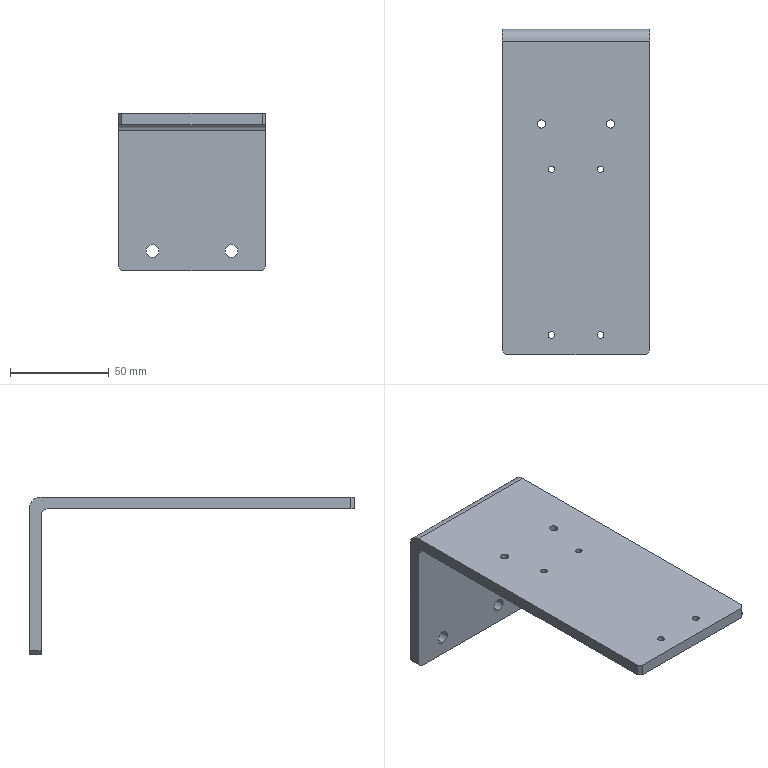Part | SolidWorks | features HoleWzd 3, Fillet 2, Chamfer 1, Extrusion 1, Shell 1 | 1 solid | 30 faces | box 75 x 165 x 80 mm | volume 106298 mm3 | cylinder 18 | plane 12 | commonest cylinder face diameters 3.3 x8 4.2 x4 6.5 x4 6 x1 12 x1
STEP:
#1=CARTESIAN_POINT('',(19.6,34.5,80.));
#2=VERTEX_POINT('',#1);
#3=CARTESIAN_POINT('',(15.4,34.5,80.));
#4=VERTEX_POINT('',#3);
#5=CARTESIAN_POINT('',(17.5,34.5,80.));
#6=DIRECTION('',(0.,0.,-1.));
#7=DIRECTION('',(-1.,0.,0.));
#8=AXIS2_PLACEMENT_3D('',#5,#6,#7);
#9=CIRCLE('',#8,2.1);
#10=EDGE_CURVE('',#2,#4,#9,.T.);
#11=ORIENTED_EDGE('',*,*,#10,.F.);
#12=CARTESIAN_POINT('',(19.6,34.5,74.));
#13=VERTEX_POINT('',#12);
#14=CARTESIAN_POINT('',(19.6,34.5,74.));
#15=DIRECTION('',(0.,0.,-1.));
#16=VECTOR('',#15,1000.);
#17=LINE('',#14,#16);
#18=EDGE_CURVE('',#2,#13,#17,.T.);
#19=ORIENTED_EDGE('',*,*,#18,.T.);
#20=CARTESIAN_POINT('',(15.4,34.5,74.));
#21=VERTEX_POINT('',#20);
#22=CARTESIAN_POINT('',(17.5,34.5,74.));
#23=DIRECTION('',(0.,0.,-1.));
#24=DIRECTION('',(-1.,0.,0.));
#25=AXIS2_PLACEMENT_3D('',#22,#23,#24);
#26=CIRCLE('',#25,2.1);
#27=EDGE_CURVE('',#13,#21,#26,.T.);
#28=ORIENTED_EDGE('',*,*,#27,.T.);
#29=CARTESIAN_POINT('',(15.4,34.5,74.));
#30=DIRECTION('',(0.,0.,-1.));
#31=VECTOR('',#30,1000.);
#32=LINE('',#29,#31);
#33=EDGE_CURVE('',#4,#21,#32,.T.);
#34=ORIENTED_EDGE('',*,*,#33,.F.);
#35=EDGE_LOOP('',(#11,#19,#28,#34));
#36=FACE_OUTER_BOUND('',#35,.T.);
#37=CARTESIAN_POINT('',(17.5,34.5,74.));
#38=DIRECTION('',(0.,0.,-1.));
#39=DIRECTION('',(-1.,0.,0.));
#40=AXIS2_PLACEMENT_3D('',#37,#38,#39);
#41=CYLINDRICAL_SURFACE('',#40,2.1);
#42=ADVANCED_FACE('',(#36),#41,.F.);
#43=CARTESIAN_POINT('',(-15.4,34.5,80.));
#44=VERTEX_POINT('',#43);
#45=CARTESIAN_POINT('',(-19.6,34.5,80.));
#46=VERTEX_POINT('',#45);
#47=CARTESIAN_POINT('',(-17.5,34.5,80.));
#48=DIRECTION('',(0.,0.,-1.));
#49=DIRECTION('',(-1.,0.,0.));
#50=AXIS2_PLACEMENT_3D('',#47,#48,#49);
#51=CIRCLE('',#50,2.1);
#52=EDGE_CURVE('',#44,#46,#51,.T.);
#53=ORIENTED_EDGE('',*,*,#52,.F.);
#54=CARTESIAN_POINT('',(-15.4,34.5,74.));
#55=VERTEX_POINT('',#54);
#56=CARTESIAN_POINT('',(-15.4,34.5,74.));
#57=DIRECTION('',(0.,0.,-1.));
#58=VECTOR('',#57,1000.);
#59=LINE('',#56,#58);
#60=EDGE_CURVE('',#44,#55,#59,.T.);
#61=ORIENTED_EDGE('',*,*,#60,.T.);
#62=CARTESIAN_POINT('',(-19.6,34.5,74.));
#63=VERTEX_POINT('',#62);
#64=CARTESIAN_POINT('',(-17.5,34.5,74.));
#65=DIRECTION('',(0.,0.,-1.));
#66=DIRECTION('',(-1.,0.,0.));
#67=AXIS2_PLACEMENT_3D('',#64,#65,#66);
#68=CIRCLE('',#67,2.1);
#69=EDGE_CURVE('',#55,#63,#68,.T.);
#70=ORIENTED_EDGE('',*,*,#69,.T.);
#71=CARTESIAN_POINT('',(-19.6,34.5,74.));
#72=DIRECTION('',(0.,0.,-1.));
#73=VECTOR('',#72,1000.);
#74=LINE('',#71,#73);
#75=EDGE_CURVE('',#46,#63,#74,.T.);
#76=ORIENTED_EDGE('',*,*,#75,.F.);
#77=EDGE_LOOP('',(#53,#61,#70,#76));
#78=FACE_OUTER_BOUND('',#77,.T.);
#79=CARTESIAN_POINT('',(-17.5,34.5,74.));
#80=DIRECTION('',(0.,0.,-1.));
#81=DIRECTION('',(-1.,0.,0.));
#82=AXIS2_PLACEMENT_3D('',#79,#80,#81);
#83=CYLINDRICAL_SURFACE('',#82,2.1);
#84=ADVANCED_FACE('',(#78),#83,.F.);
#85=CARTESIAN_POINT('',(-20.,82.5,13.25));
#86=VERTEX_POINT('',#85);
#87=CARTESIAN_POINT('',(-20.,82.5,6.75));
#88=VERTEX_POINT('',#87);
#89=CARTESIAN_POINT('',(-20.,82.5,10.));
#90=DIRECTION('',(0.,-1.,0.));
#91=DIRECTION('',(0.,0.,-1.));
#92=AXIS2_PLACEMENT_3D('',#89,#90,#91);
#93=CIRCLE('',#92,3.25);
#94=EDGE_CURVE('',#86,#88,#93,.T.);
#95=ORIENTED_EDGE('',*,*,#94,.F.);
#96=CARTESIAN_POINT('',(-20.,76.5,13.25));
#97=VERTEX_POINT('',#96);
#98=CARTESIAN_POINT('',(-20.,76.5,13.25));
#99=DIRECTION('',(0.,-1.,0.));
#100=VECTOR('',#99,1000.);
#101=LINE('',#98,#100);
#102=EDGE_CURVE('',#86,#97,#101,.T.);
#103=ORIENTED_EDGE('',*,*,#102,.T.);
#104=CARTESIAN_POINT('',(-20.,76.5,6.75));
#105=VERTEX_POINT('',#104);
#106=CARTESIAN_POINT('',(-20.,76.5,10.));
#107=DIRECTION('',(0.,-1.,0.));
#108=DIRECTION('',(0.,0.,-1.));
#109=AXIS2_PLACEMENT_3D('',#106,#107,#108);
#110=CIRCLE('',#109,3.25);
#111=EDGE_CURVE('',#97,#105,#110,.T.);
#112=ORIENTED_EDGE('',*,*,#111,.T.);
#113=CARTESIAN_POINT('',(-20.,76.5,6.75));
#114=DIRECTION('',(0.,-1.,0.));
#115=VECTOR('',#114,1000.);
#116=LINE('',#113,#115);
#117=EDGE_CURVE('',#88,#105,#116,.T.);
#118=ORIENTED_EDGE('',*,*,#117,.F.);
#119=EDGE_LOOP('',(#95,#103,#112,#118));
#120=FACE_OUTER_BOUND('',#119,.T.);
#121=CARTESIAN_POINT('',(-20.,76.5,10.));
#122=DIRECTION('',(0.,-1.,0.));
#123=DIRECTION('',(0.,0.,-1.));
#124=AXIS2_PLACEMENT_3D('',#121,#122,#123);
#125=CYLINDRICAL_SURFACE('',#124,3.25);
#126=ADVANCED_FACE('',(#120),#125,.F.);
#127=CARTESIAN_POINT('',(20.,82.5,13.25));
#128=VERTEX_POINT('',#127);
#129=CARTESIAN_POINT('',(20.,82.5,6.75));
#130=VERTEX_POINT('',#129);
#131=CARTESIAN_POINT('',(20.,82.5,10.));
#132=DIRECTION('',(0.,-1.,0.));
#133=DIRECTION('',(0.,0.,-1.));
#134=AXIS2_PLACEMENT_3D('',#131,#132,#133);
#135=CIRCLE('',#134,3.25);
#136=EDGE_CURVE('',#128,#130,#135,.T.);
#137=ORIENTED_EDGE('',*,*,#136,.F.);
#138=CARTESIAN_POINT('',(20.,76.5,13.25));
#139=VERTEX_POINT('',#138);
#140=CARTESIAN_POINT('',(20.,76.5,13.25));
#141=DIRECTION('',(0.,-1.,0.));
#142=VECTOR('',#141,1000.);
#143=LINE('',#140,#142);
#144=EDGE_CURVE('',#128,#139,#143,.T.);
#145=ORIENTED_EDGE('',*,*,#144,.T.);
#146=CARTESIAN_POINT('',(20.,76.5,6.75));
#147=VERTEX_POINT('',#146);
#148=CARTESIAN_POINT('',(20.,76.5,10.));
#149=DIRECTION('',(0.,-1.,0.));
#150=DIRECTION('',(0.,0.,-1.));
#151=AXIS2_PLACEMENT_3D('',#148,#149,#150);
#152=CIRCLE('',#151,3.25);
#153=EDGE_CURVE('',#139,#147,#152,.T.);
#154=ORIENTED_EDGE('',*,*,#153,.T.);
#155=CARTESIAN_POINT('',(20.,76.5,6.75));
#156=DIRECTION('',(0.,-1.,0.));
#157=VECTOR('',#156,1000.);
#158=LINE('',#155,#157);
#159=EDGE_CURVE('',#130,#147,#158,.T.);
#160=ORIENTED_EDGE('',*,*,#159,.F.);
#161=EDGE_LOOP('',(#137,#145,#154,#160));
#162=FACE_OUTER_BOUND('',#161,.T.);
#163=CARTESIAN_POINT('',(20.,76.5,10.));
#164=DIRECTION('',(0.,-1.,0.));
#165=DIRECTION('',(0.,0.,-1.));
#166=AXIS2_PLACEMENT_3D('',#163,#164,#165);
#167=CYLINDRICAL_SURFACE('',#166,3.25);
#168=ADVANCED_FACE('',(#162),#167,.F.);
#169=CARTESIAN_POINT('',(14.15,-72.5,80.));
#170=VERTEX_POINT('',#169);
#171=CARTESIAN_POINT('',(10.85,-72.5,80.));
#172=VERTEX_POINT('',#171);
#173=CARTESIAN_POINT('',(12.5,-72.5,80.));
#174=DIRECTION('',(0.,0.,-1.));
#175=DIRECTION('',(-1.,0.,0.));
#176=AXIS2_PLACEMENT_3D('',#173,#174,#175);
#177=CIRCLE('',#176,1.65);
#178=EDGE_CURVE('',#170,#172,#177,.T.);
#179=ORIENTED_EDGE('',*,*,#178,.F.);
#180=CARTESIAN_POINT('',(14.15,-72.5,74.));
#181=VERTEX_POINT('',#180);
#182=CARTESIAN_POINT('',(14.15,-72.5,74.));
#183=DIRECTION('',(0.,0.,-1.));
#184=VECTOR('',#183,1000.);
#185=LINE('',#182,#184);
#186=EDGE_CURVE('',#170,#181,#185,.T.);
#187=ORIENTED_EDGE('',*,*,#186,.T.);
#188=CARTESIAN_POINT('',(10.85,-72.5,74.));
#189=VERTEX_POINT('',#188);
#190=CARTESIAN_POINT('',(12.5,-72.5,74.));
#191=DIRECTION('',(0.,0.,-1.));
#192=DIRECTION('',(-1.,0.,0.));
#193=AXIS2_PLACEMENT_3D('',#190,#191,#192);
#194=CIRCLE('',#193,1.65);
#195=EDGE_CURVE('',#181,#189,#194,.T.);
#196=ORIENTED_EDGE('',*,*,#195,.T.);
#197=CARTESIAN_POINT('',(10.85,-72.5,74.));
#198=DIRECTION('',(0.,0.,-1.));
#199=VECTOR('',#198,1000.);
#200=LINE('',#197,#199);
#201=EDGE_CURVE('',#172,#189,#200,.T.);
#202=ORIENTED_EDGE('',*,*,#201,.F.);
#203=EDGE_LOOP('',(#179,#187,#196,#202));
#204=FACE_OUTER_BOUND('',#203,.T.);
#205=CARTESIAN_POINT('',(12.5,-72.5,74.));
#206=DIRECTION('',(0.,0.,-1.));
#207=DIRECTION('',(-1.,0.,0.));
#208=AXIS2_PLACEMENT_3D('',#205,#206,#207);
#209=CYLINDRICAL_SURFACE('',#208,1.65);
#210=ADVANCED_FACE('',(#204),#209,.F.);
#211=CARTESIAN_POINT('',(14.15,11.5,80.));
#212=VERTEX_POINT('',#211);
#213=CARTESIAN_POINT('',(10.85,11.5,80.));
#214=VERTEX_POINT('',#213);
#215=CARTESIAN_POINT('',(12.5,11.5,80.));
#216=DIRECTION('',(0.,0.,-1.));
#217=DIRECTION('',(-1.,0.,0.));
#218=AXIS2_PLACEMENT_3D('',#215,#216,#217);
#219=CIRCLE('',#218,1.65);
#220=EDGE_CURVE('',#212,#214,#219,.T.);
#221=ORIENTED_EDGE('',*,*,#220,.F.);
#222=CARTESIAN_POINT('',(14.15,11.5,74.));
#223=VERTEX_POINT('',#222);
#224=CARTESIAN_POINT('',(14.15,11.5,74.));
#225=DIRECTION('',(0.,0.,-1.));
#226=VECTOR('',#225,1000.);
#227=LINE('',#224,#226);
#228=EDGE_CURVE('',#212,#223,#227,.T.);
#229=ORIENTED_EDGE('',*,*,#228,.T.);
#230=CARTESIAN_POINT('',(10.85,11.5,74.));
#231=VERTEX_POINT('',#230);
#232=CARTESIAN_POINT('',(12.5,11.5,74.));
#233=DIRECTION('',(0.,0.,-1.));
#234=DIRECTION('',(-1.,0.,0.));
#235=AXIS2_PLACEMENT_3D('',#232,#233,#234);
#236=CIRCLE('',#235,1.65);
#237=EDGE_CURVE('',#223,#231,#236,.T.);
#238=ORIENTED_EDGE('',*,*,#237,.T.);
#239=CARTESIAN_POINT('',(10.85,11.5,74.));
#240=DIRECTION('',(0.,0.,-1.));
#241=VECTOR('',#240,1000.);
#242=LINE('',#239,#241);
#243=EDGE_CURVE('',#214,#231,#242,.T.);
#244=ORIENTED_EDGE('',*,*,#243,.F.);
#245=EDGE_LOOP('',(#221,#229,#238,#244));
#246=FACE_OUTER_BOUND('',#245,.T.);
#247=CARTESIAN_POINT('',(12.5,11.5,74.));
#248=DIRECTION('',(0.,0.,-1.));
#249=DIRECTION('',(-1.,0.,0.));
#250=AXIS2_PLACEMENT_3D('',#247,#248,#249);
#251=CYLINDRICAL_SURFACE('',#250,1.65);
#252=ADVANCED_FACE('',(#246),#251,.F.);
#253=CARTESIAN_POINT('',(-10.85,11.5,80.));
#254=VERTEX_POINT('',#253);
#255=CARTESIAN_POINT('',(-14.15,11.5,80.));
#256=VERTEX_POINT('',#255);
#257=CARTESIAN_POINT('',(-12.5,11.5,80.));
#258=DIRECTION('',(0.,0.,-1.));
#259=DIRECTION('',(-1.,0.,0.));
#260=AXIS2_PLACEMENT_3D('',#257,#258,#259);
#261=CIRCLE('',#260,1.65);
#262=EDGE_CURVE('',#254,#256,#261,.T.);
#263=ORIENTED_EDGE('',*,*,#262,.F.);
#264=CARTESIAN_POINT('',(-10.85,11.5,74.));
#265=VERTEX_POINT('',#264);
#266=CARTESIAN_POINT('',(-10.85,11.5,74.));
#267=DIRECTION('',(0.,0.,-1.));
#268=VECTOR('',#267,1000.);
#269=LINE('',#266,#268);
#270=EDGE_CURVE('',#254,#265,#269,.T.);
#271=ORIENTED_EDGE('',*,*,#270,.T.);
#272=CARTESIAN_POINT('',(-14.15,11.5,74.));
#273=VERTEX_POINT('',#272);
#274=CARTESIAN_POINT('',(-12.5,11.5,74.));
#275=DIRECTION('',(0.,0.,-1.));
#276=DIRECTION('',(-1.,0.,0.));
#277=AXIS2_PLACEMENT_3D('',#274,#275,#276);
#278=CIRCLE('',#277,1.65);
#279=EDGE_CURVE('',#265,#273,#278,.T.);
#280=ORIENTED_EDGE('',*,*,#279,.T.);
#281=CARTESIAN_POINT('',(-14.15,11.5,74.));
#282=DIRECTION('',(0.,0.,-1.));
#283=VECTOR('',#282,1000.);
#284=LINE('',#281,#283);
#285=EDGE_CURVE('',#256,#273,#284,.T.);
#286=ORIENTED_EDGE('',*,*,#285,.F.);
#287=EDGE_LOOP('',(#263,#271,#280,#286));
#288=FACE_OUTER_BOUND('',#287,.T.);
#289=CARTESIAN_POINT('',(-12.5,11.5,74.));
#290=DIRECTION('',(0.,0.,-1.));
#291=DIRECTION('',(-1.,0.,0.));
#292=AXIS2_PLACEMENT_3D('',#289,#290,#291);
#293=CYLINDRICAL_SURFACE('',#292,1.65);
#294=ADVANCED_FACE('',(#288),#293,.F.);
#295=CARTESIAN_POINT('',(-10.85,-72.5,80.));
#296=VERTEX_POINT('',#295);
#297=CARTESIAN_POINT('',(-14.15,-72.5,80.));
#298=VERTEX_POINT('',#297);
#299=CARTESIAN_POINT('',(-12.5,-72.5,80.));
#300=DIRECTION('',(0.,0.,-1.));
#301=DIRECTION('',(-1.,0.,0.));
#302=AXIS2_PLACEMENT_3D('',#299,#300,#301);
#303=CIRCLE('',#302,1.65);
#304=EDGE_CURVE('',#296,#298,#303,.T.);
#305=ORIENTED_EDGE('',*,*,#304,.F.);
#306=CARTESIAN_POINT('',(-10.85,-72.5,74.));
#307=VERTEX_POINT('',#306);
#308=CARTESIAN_POINT('',(-10.85,-72.5,74.));
#309=DIRECTION('',(0.,0.,-1.));
#310=VECTOR('',#309,1000.);
#311=LINE('',#308,#310);
#312=EDGE_CURVE('',#296,#307,#311,.T.);
#313=ORIENTED_EDGE('',*,*,#312,.T.);
#314=CARTESIAN_POINT('',(-14.15,-72.5,74.));
#315=VERTEX_POINT('',#314);
#316=CARTESIAN_POINT('',(-12.5,-72.5,74.));
#317=DIRECTION('',(0.,0.,-1.));
#318=DIRECTION('',(-1.,0.,0.));
#319=AXIS2_PLACEMENT_3D('',#316,#317,#318);
#320=CIRCLE('',#319,1.65);
#321=EDGE_CURVE('',#307,#315,#320,.T.);
#322=ORIENTED_EDGE('',*,*,#321,.T.);
#323=CARTESIAN_POINT('',(-14.15,-72.5,74.));
#324=DIRECTION('',(0.,0.,-1.));
#325=VECTOR('',#324,1000.);
#326=LINE('',#323,#325);
#327=EDGE_CURVE('',#298,#315,#326,.T.);
#328=ORIENTED_EDGE('',*,*,#327,.F.);
#329=EDGE_LOOP('',(#305,#313,#322,#328));
#330=FACE_OUTER_BOUND('',#329,.T.);
#331=CARTESIAN_POINT('',(-12.5,-72.5,74.));
#332=DIRECTION('',(0.,0.,-1.));
#333=DIRECTION('',(-1.,0.,0.));
#334=AXIS2_PLACEMENT_3D('',#331,#332,#333);
#335=CYLINDRICAL_SURFACE('',#334,1.65);
#336=ADVANCED_FACE('',(#330),#335,.F.);
#337=CARTESIAN_POINT('',(37.5,-80.5,80.));
#338=VERTEX_POINT('',#337);
#339=CARTESIAN_POINT('',(37.5,76.5,80.));
#340=VERTEX_POINT('',#339);
#341=CARTESIAN_POINT('',(37.5,82.5,80.));
#342=DIRECTION('',(0.,1.,0.));
#343=VECTOR('',#342,1000.);
#344=LINE('',#341,#343);
#345=EDGE_CURVE('',#338,#340,#344,.T.);
#346=ORIENTED_EDGE('',*,*,#345,.F.);
#347=CARTESIAN_POINT('',(37.5,-80.5,74.));
#348=VERTEX_POINT('',#347);
#349=CARTESIAN_POINT('',(37.5,-80.5,80.));
#350=DIRECTION('',(0.,0.,-1.));
#351=VECTOR('',#350,1000.);
#352=LINE('',#349,#351);
#353=EDGE_CURVE('',#338,#348,#352,.T.);
#354=ORIENTED_EDGE('',*,*,#353,.T.);
#355=CARTESIAN_POINT('',(37.5,73.5,74.));
#356=VERTEX_POINT('',#355);
#357=CARTESIAN_POINT('',(37.5,82.5,74.));
#358=DIRECTION('',(0.,1.,0.));
#359=VECTOR('',#358,1000.);
#360=LINE('',#357,#359);
#361=EDGE_CURVE('',#348,#356,#360,.T.);
#362=ORIENTED_EDGE('',*,*,#361,.T.);
#363=CARTESIAN_POINT('',(37.5,76.5,71.));
#364=VERTEX_POINT('',#363);
#365=CARTESIAN_POINT('',(37.5,73.5,71.));
#366=DIRECTION('',(-1.,0.,0.));
#367=DIRECTION('',(0.,-1.,0.));
#368=AXIS2_PLACEMENT_3D('',#365,#366,#367);
#369=CIRCLE('',#368,3.);
#370=EDGE_CURVE('',#356,#364,#369,.T.);
#371=ORIENTED_EDGE('',*,*,#370,.T.);
#372=CARTESIAN_POINT('',(37.5,76.5,2.));
#373=VERTEX_POINT('',#372);
#374=CARTESIAN_POINT('',(37.5,76.5,80.));
#375=DIRECTION('',(0.,0.,-1.));
#376=VECTOR('',#375,1000.);
#377=LINE('',#374,#376);
#378=EDGE_CURVE('',#364,#373,#377,.T.);
#379=ORIENTED_EDGE('',*,*,#378,.T.);
#380=CARTESIAN_POINT('',(37.5,82.5,2.));
#381=VERTEX_POINT('',#380);
#382=CARTESIAN_POINT('',(37.5,82.5,2.));
#383=DIRECTION('',(0.,1.,0.));
#384=VECTOR('',#383,1000.);
#385=LINE('',#382,#384);
#386=EDGE_CURVE('',#373,#381,#385,.T.);
#387=ORIENTED_EDGE('',*,*,#386,.T.);
#388=CARTESIAN_POINT('',(37.5,82.5,74.));
#389=VERTEX_POINT('',#388);
#390=CARTESIAN_POINT('',(37.5,82.5,80.));
#391=DIRECTION('',(0.,0.,-1.));
#392=VECTOR('',#391,1000.);
#393=LINE('',#390,#392);
#394=EDGE_CURVE('',#389,#381,#393,.T.);
#395=ORIENTED_EDGE('',*,*,#394,.F.);
#396=CARTESIAN_POINT('',(37.5,76.5,74.));
#397=DIRECTION('',(1.,0.,0.));
#398=DIRECTION('',(0.,-1.,0.));
#399=AXIS2_PLACEMENT_3D('',#396,#397,#398);
#400=CIRCLE('',#399,6.);
#401=EDGE_CURVE('',#389,#340,#400,.T.);
#402=ORIENTED_EDGE('',*,*,#401,.T.);
#403=EDGE_LOOP('',(#346,#354,#362,#371,#379,#387,#395,#402));
#404=FACE_OUTER_BOUND('',#403,.T.);
#405=CARTESIAN_POINT('',(37.5,82.5,80.));
#406=DIRECTION('',(-1.,0.,0.));
#407=DIRECTION('',(0.,-1.,0.));
#408=AXIS2_PLACEMENT_3D('',#405,#406,#407);
#409=PLANE('',#408);
#410=ADVANCED_FACE('',(#404),#409,.F.);
#411=CARTESIAN_POINT('',(-20.,82.5,10.));
#412=DIRECTION('',(0.,-1.,0.));
#413=DIRECTION('',(0.,0.,-1.));
#414=AXIS2_PLACEMENT_3D('',#411,#412,#413);
#415=CIRCLE('',#414,3.25);
#416=EDGE_CURVE('',#88,#86,#415,.T.);
#417=ORIENTED_EDGE('',*,*,#416,.T.);
#418=ORIENTED_EDGE('',*,*,#94,.T.);
#419=EDGE_LOOP('',(#417,#418));
#420=FACE_BOUND('',#419,.T.);
#421=CARTESIAN_POINT('',(20.,82.5,10.));
#422=DIRECTION('',(0.,-1.,0.));
#423=DIRECTION('',(0.,0.,-1.));
#424=AXIS2_PLACEMENT_3D('',#421,#422,#423);
#425=CIRCLE('',#424,3.25);
#426=EDGE_CURVE('',#130,#128,#425,.T.);
#427=ORIENTED_EDGE('',*,*,#426,.T.);
#428=ORIENTED_EDGE('',*,*,#136,.T.);
#429=EDGE_LOOP('',(#427,#428));
#430=FACE_BOUND('',#429,.T.);
#431=CARTESIAN_POINT('',(35.5,82.5,0.));
#432=VERTEX_POINT('',#431);
#433=CARTESIAN_POINT('',(-35.5,82.5,0.));
#434=VERTEX_POINT('',#433);
#435=CARTESIAN_POINT('',(-37.5,82.5,0.));
#436=DIRECTION('',(-1.,0.,0.));
#437=VECTOR('',#436,1000.);
#438=LINE('',#435,#437);
#439=EDGE_CURVE('',#432,#434,#438,.T.);
#440=ORIENTED_EDGE('',*,*,#439,.T.);
#441=CARTESIAN_POINT('',(-37.5,82.5,2.));
#442=VERTEX_POINT('',#441);
#443=CARTESIAN_POINT('',(-37.5,82.5,2.));
#444=DIRECTION('',(-0.7071,0.,0.7071));
#445=VECTOR('',#444,1000.);
#446=LINE('',#443,#445);
#447=EDGE_CURVE('',#434,#442,#446,.T.);
#448=ORIENTED_EDGE('',*,*,#447,.T.);
#449=CARTESIAN_POINT('',(-37.5,82.5,74.));
#450=VERTEX_POINT('',#449);
#451=CARTESIAN_POINT('',(-37.5,82.5,80.));
#452=DIRECTION('',(0.,0.,-1.));
#453=VECTOR('',#452,1000.);
#454=LINE('',#451,#453);
#455=EDGE_CURVE('',#450,#442,#454,.T.);
#456=ORIENTED_EDGE('',*,*,#455,.F.);
#457=CARTESIAN_POINT('',(37.5,82.5,74.));
#458=DIRECTION('',(1.,0.,0.));
#459=VECTOR('',#458,1000.);
#460=LINE('',#457,#459);
#461=EDGE_CURVE('',#450,#389,#460,.T.);
#462=ORIENTED_EDGE('',*,*,#461,.T.);
#463=ORIENTED_EDGE('',*,*,#394,.T.);
#464=CARTESIAN_POINT('',(37.5,82.5,2.));
#465=DIRECTION('',(-0.7071,0.,-0.7071));
#466=VECTOR('',#465,1000.);
#467=LINE('',#464,#466);
#468=EDGE_CURVE('',#381,#432,#467,.T.);
#469=ORIENTED_EDGE('',*,*,#468,.T.);
#470=EDGE_LOOP('',(#440,#448,#456,#462,#463,#469));
#471=FACE_OUTER_BOUND('',#470,.T.);
#472=CARTESIAN_POINT('',(-37.5,82.5,80.));
#473=DIRECTION('',(0.,-1.,0.));
#474=DIRECTION('',(0.,0.,-1.));
#475=AXIS2_PLACEMENT_3D('',#472,#473,#474);
#476=PLANE('',#475);
#477=ADVANCED_FACE('',(#420,#430,#471),#476,.F.);
#478=CARTESIAN_POINT('',(-37.5,73.5,74.));
#479=VERTEX_POINT('',#478);
#480=CARTESIAN_POINT('',(-37.5,-80.5,74.));
#481=VERTEX_POINT('',#480);
#482=CARTESIAN_POINT('',(-37.5,82.5,74.));
#483=DIRECTION('',(0.,-1.,0.));
#484=VECTOR('',#483,1000.);
#485=LINE('',#482,#484);
#486=EDGE_CURVE('',#479,#481,#485,.T.);
#487=ORIENTED_EDGE('',*,*,#486,.T.);
#488=CARTESIAN_POINT('',(-37.5,-80.5,80.));
#489=VERTEX_POINT('',#488);
#490=CARTESIAN_POINT('',(-37.5,-80.5,80.));
#491=DIRECTION('',(0.,0.,1.));
#492=VECTOR('',#491,1000.);
#493=LINE('',#490,#492);
#494=EDGE_CURVE('',#481,#489,#493,.T.);
#495=ORIENTED_EDGE('',*,*,#494,.T.);
#496=CARTESIAN_POINT('',(-37.5,76.5,80.));
#497=VERTEX_POINT('',#496);
#498=CARTESIAN_POINT('',(-37.5,82.5,80.));
#499=DIRECTION('',(0.,-1.,0.));
#500=VECTOR('',#499,1000.);
#501=LINE('',#498,#500);
#502=EDGE_CURVE('',#497,#489,#501,.T.);
#503=ORIENTED_EDGE('',*,*,#502,.F.);
#504=CARTESIAN_POINT('',(-37.5,76.5,74.));
#505=DIRECTION('',(-1.,0.,0.));
#506=DIRECTION('',(0.,1.,0.));
#507=AXIS2_PLACEMENT_3D('',#504,#505,#506);
#508=CIRCLE('',#507,6.);
#509=EDGE_CURVE('',#497,#450,#508,.T.);
#510=ORIENTED_EDGE('',*,*,#509,.T.);
#511=ORIENTED_EDGE('',*,*,#455,.T.);
#512=CARTESIAN_POINT('',(-37.5,76.5,2.));
#513=VERTEX_POINT('',#512);
#514=CARTESIAN_POINT('',(-37.5,82.5,2.));
#515=DIRECTION('',(0.,-1.,0.));
#516=VECTOR('',#515,1000.);
#517=LINE('',#514,#516);
#518=EDGE_CURVE('',#442,#513,#517,.T.);
#519=ORIENTED_EDGE('',*,*,#518,.T.);
#520=CARTESIAN_POINT('',(-37.5,76.5,71.));
#521=VERTEX_POINT('',#520);
#522=CARTESIAN_POINT('',(-37.5,76.5,80.));
#523=DIRECTION('',(0.,0.,-1.));
#524=VECTOR('',#523,1000.);
#525=LINE('',#522,#524);
#526=EDGE_CURVE('',#521,#513,#525,.T.);
#527=ORIENTED_EDGE('',*,*,#526,.F.);
#528=CARTESIAN_POINT('',(-37.5,73.5,71.));
#529=DIRECTION('',(1.,0.,0.));
#530=DIRECTION('',(0.,1.,0.));
#531=AXIS2_PLACEMENT_3D('',#528,#529,#530);
#532=CIRCLE('',#531,3.);
#533=EDGE_CURVE('',#521,#479,#532,.T.);
#534=ORIENTED_EDGE('',*,*,#533,.T.);
#535=EDGE_LOOP('',(#487,#495,#503,#510,#511,#519,#527,#534));
#536=FACE_OUTER_BOUND('',#535,.T.);
#537=CARTESIAN_POINT('',(-37.5,82.5,80.));
#538=DIRECTION('',(1.,0.,0.));
#539=DIRECTION('',(0.,1.,0.));
#540=AXIS2_PLACEMENT_3D('',#537,#538,#539);
#541=PLANE('',#540);
#542=ADVANCED_FACE('',(#536),#541,.F.);
#543=CARTESIAN_POINT('',(-35.5,-82.5,74.));
#544=VERTEX_POINT('',#543);
#545=CARTESIAN_POINT('',(35.5,-82.5,74.));
#546=VERTEX_POINT('',#545);
#547=CARTESIAN_POINT('',(-37.5,-82.5,74.));
#548=DIRECTION('',(1.,0.,0.));
#549=VECTOR('',#548,1000.);
#550=LINE('',#547,#549);
#551=EDGE_CURVE('',#544,#546,#550,.T.);
#552=ORIENTED_EDGE('',*,*,#551,.T.);
#553=CARTESIAN_POINT('',(35.5,-82.5,80.));
#554=VERTEX_POINT('',#553);
#555=CARTESIAN_POINT('',(35.5,-82.5,80.));
#556=DIRECTION('',(0.,0.,1.));
#557=VECTOR('',#556,1000.);
#558=LINE('',#555,#557);
#559=EDGE_CURVE('',#546,#554,#558,.T.);
#560=ORIENTED_EDGE('',*,*,#559,.T.);
#561=CARTESIAN_POINT('',(-35.5,-82.5,80.));
#562=VERTEX_POINT('',#561);
#563=CARTESIAN_POINT('',(-37.5,-82.5,80.));
#564=DIRECTION('',(1.,0.,0.));
#565=VECTOR('',#564,1000.);
#566=LINE('',#563,#565);
#567=EDGE_CURVE('',#562,#554,#566,.T.);
#568=ORIENTED_EDGE('',*,*,#567,.F.);
#569=CARTESIAN_POINT('',(-35.5,-82.5,80.));
#570=DIRECTION('',(0.,0.,-1.));
#571=VECTOR('',#570,1000.);
#572=LINE('',#569,#571);
#573=EDGE_CURVE('',#562,#544,#572,.T.);
#574=ORIENTED_EDGE('',*,*,#573,.T.);
#575=EDGE_LOOP('',(#552,#560,#568,#574));
#576=FACE_OUTER_BOUND('',#575,.T.);
#577=CARTESIAN_POINT('',(-37.5,-82.5,80.));
#578=DIRECTION('',(0.,1.,0.));
#579=DIRECTION('',(0.,0.,1.));
#580=AXIS2_PLACEMENT_3D('',#577,#578,#579);
#581=PLANE('',#580);
#582=ADVANCED_FACE('',(#576),#581,.F.);
#583=CARTESIAN_POINT('',(17.5,34.5,80.));
#584=DIRECTION('',(0.,0.,-1.));
#585=DIRECTION('',(-1.,0.,0.));
#586=AXIS2_PLACEMENT_3D('',#583,#584,#585);
#587=CIRCLE('',#586,2.1);
#588=EDGE_CURVE('',#4,#2,#587,.T.);
#589=ORIENTED_EDGE('',*,*,#588,.T.);
#590=ORIENTED_EDGE('',*,*,#10,.T.);
#591=EDGE_LOOP('',(#589,#590));
#592=FACE_BOUND('',#591,.T.);
#593=CARTESIAN_POINT('',(-17.5,34.5,80.));
#594=DIRECTION('',(0.,0.,-1.));
#595=DIRECTION('',(-1.,0.,0.));
#596=AXIS2_PLACEMENT_3D('',#593,#594,#595);
#597=CIRCLE('',#596,2.1);
#598=EDGE_CURVE('',#46,#44,#597,.T.);
#599=ORIENTED_EDGE('',*,*,#598,.T.);
#600=ORIENTED_EDGE('',*,*,#52,.T.);
#601=EDGE_LOOP('',(#599,#600));
#602=FACE_BOUND('',#601,.T.);
#603=CARTESIAN_POINT('',(12.5,-72.5,80.));
#604=DIRECTION('',(0.,0.,-1.));
#605=DIRECTION('',(-1.,0.,0.));
#606=AXIS2_PLACEMENT_3D('',#603,#604,#605);
#607=CIRCLE('',#606,1.65);
#608=EDGE_CURVE('',#172,#170,#607,.T.);
#609=ORIENTED_EDGE('',*,*,#608,.T.);
#610=ORIENTED_EDGE('',*,*,#178,.T.);
#611=EDGE_LOOP('',(#609,#610));
#612=FACE_BOUND('',#611,.T.);
#613=CARTESIAN_POINT('',(12.5,11.5,80.));
#614=DIRECTION('',(0.,0.,-1.));
#615=DIRECTION('',(-1.,0.,0.));
#616=AXIS2_PLACEMENT_3D('',#613,#614,#615);
#617=CIRCLE('',#616,1.65);
#618=EDGE_CURVE('',#214,#212,#617,.T.);
#619=ORIENTED_EDGE('',*,*,#618,.T.);
#620=ORIENTED_EDGE('',*,*,#220,.T.);
#621=EDGE_LOOP('',(#619,#620));
#622=FACE_BOUND('',#621,.T.);
#623=CARTESIAN_POINT('',(-12.5,11.5,80.));
#624=DIRECTION('',(0.,0.,-1.));
#625=DIRECTION('',(-1.,0.,0.));
#626=AXIS2_PLACEMENT_3D('',#623,#624,#625);
#627=CIRCLE('',#626,1.65);
#628=EDGE_CURVE('',#256,#254,#627,.T.);
#629=ORIENTED_EDGE('',*,*,#628,.T.);
#630=ORIENTED_EDGE('',*,*,#262,.T.);
#631=EDGE_LOOP('',(#629,#630));
#632=FACE_BOUND('',#631,.T.);
#633=CARTESIAN_POINT('',(-12.5,-72.5,80.));
#634=DIRECTION('',(0.,0.,-1.));
#635=DIRECTION('',(-1.,0.,0.));
#636=AXIS2_PLACEMENT_3D('',#633,#634,#635);
#637=CIRCLE('',#636,1.65);
#638=EDGE_CURVE('',#298,#296,#637,.T.);
#639=ORIENTED_EDGE('',*,*,#638,.T.);
#640=ORIENTED_EDGE('',*,*,#304,.T.);
#641=EDGE_LOOP('',(#639,#640));
#642=FACE_BOUND('',#641,.T.);
#643=ORIENTED_EDGE('',*,*,#567,.T.);
#644=CARTESIAN_POINT('',(36.5,-81.5,80.));
#645=DIRECTION('',(0.7071,0.7071,0.));
#646=VECTOR('',#645,1000.);
#647=LINE('',#644,#646);
#648=EDGE_CURVE('',#554,#338,#647,.T.);
#649=ORIENTED_EDGE('',*,*,#648,.T.);
#650=ORIENTED_EDGE('',*,*,#345,.T.);
#651=CARTESIAN_POINT('',(-37.5,76.5,80.));
#652=DIRECTION('',(-1.,0.,0.));
#653=VECTOR('',#652,1000.);
#654=LINE('',#651,#653);
#655=EDGE_CURVE('',#340,#497,#654,.T.);
#656=ORIENTED_EDGE('',*,*,#655,.T.);
#657=ORIENTED_EDGE('',*,*,#502,.T.);
#658=CARTESIAN_POINT('',(1.,-119.,80.));
#659=DIRECTION('',(0.7071,-0.7071,0.));
#660=VECTOR('',#659,1000.);
#661=LINE('',#658,#660);
#662=EDGE_CURVE('',#489,#562,#661,.T.);
#663=ORIENTED_EDGE('',*,*,#662,.T.);
#664=EDGE_LOOP('',(#643,#649,#650,#656,#657,#663));
#665=FACE_OUTER_BOUND('',#664,.T.);
#666=CARTESIAN_POINT('',(37.5,-82.5,80.));
#667=DIRECTION('',(0.,0.,1.));
#668=DIRECTION('',(1.,0.,0.));
#669=AXIS2_PLACEMENT_3D('',#666,#667,#668);
#670=PLANE('',#669);
#671=ADVANCED_FACE('',(#592,#602,#612,#622,#632,#642,#665),#670,.T.);
#672=CARTESIAN_POINT('',(35.5,76.5,0.));
#673=VERTEX_POINT('',#672);
#674=CARTESIAN_POINT('',(-35.5,76.5,0.));
#675=VERTEX_POINT('',#674);
#676=CARTESIAN_POINT('',(-37.5,76.5,0.));
#677=DIRECTION('',(-1.,0.,0.));
#678=VECTOR('',#677,1000.);
#679=LINE('',#676,#678);
#680=EDGE_CURVE('',#673,#675,#679,.T.);
#681=ORIENTED_EDGE('',*,*,#680,.T.);
#682=CARTESIAN_POINT('',(-35.5,-82.5,0.));
#683=DIRECTION('',(0.,1.,0.));
#684=VECTOR('',#683,1000.);
#685=LINE('',#682,#684);
#686=EDGE_CURVE('',#675,#434,#685,.T.);
#687=ORIENTED_EDGE('',*,*,#686,.T.);
#688=ORIENTED_EDGE('',*,*,#439,.F.);
#689=CARTESIAN_POINT('',(35.5,-82.5,0.));
#690=DIRECTION('',(0.,-1.,0.));
#691=VECTOR('',#690,1000.);
#692=LINE('',#689,#691);
#693=EDGE_CURVE('',#432,#673,#692,.T.);
#694=ORIENTED_EDGE('',*,*,#693,.T.);
#695=EDGE_LOOP('',(#681,#687,#688,#694));
#696=FACE_OUTER_BOUND('',#695,.T.);
#697=CARTESIAN_POINT('',(37.5,-82.5,0.));
#698=DIRECTION('',(0.,0.,1.));
#699=DIRECTION('',(1.,0.,0.));
#700=AXIS2_PLACEMENT_3D('',#697,#698,#699);
#701=PLANE('',#700);
#702=ADVANCED_FACE('',(#696),#701,.F.);
#703=CARTESIAN_POINT('',(-20.,76.5,10.));
#704=DIRECTION('',(0.,-1.,0.));
#705=DIRECTION('',(0.,0.,-1.));
#706=AXIS2_PLACEMENT_3D('',#703,#704,#705);
#707=CIRCLE('',#706,3.25);
#708=EDGE_CURVE('',#105,#97,#707,.T.);
#709=ORIENTED_EDGE('',*,*,#708,.F.);
#710=ORIENTED_EDGE('',*,*,#111,.F.);
#711=EDGE_LOOP('',(#709,#710));
#712=FACE_BOUND('',#711,.T.);
#713=CARTESIAN_POINT('',(20.,76.5,10.));
#714=DIRECTION('',(0.,-1.,0.));
#715=DIRECTION('',(0.,0.,-1.));
#716=AXIS2_PLACEMENT_3D('',#713,#714,#715);
#717=CIRCLE('',#716,3.25);
#718=EDGE_CURVE('',#147,#139,#717,.T.);
#719=ORIENTED_EDGE('',*,*,#718,.F.);
#720=ORIENTED_EDGE('',*,*,#153,.F.);
#721=EDGE_LOOP('',(#719,#720));
#722=FACE_BOUND('',#721,.T.);
#723=ORIENTED_EDGE('',*,*,#526,.T.);
#724=CARTESIAN_POINT('',(-76.5,76.5,41.));
#725=DIRECTION('',(0.7071,0.,-0.7071));
#726=VECTOR('',#725,1000.);
#727=LINE('',#724,#726);
#728=EDGE_CURVE('',#513,#675,#727,.T.);
#729=ORIENTED_EDGE('',*,*,#728,.T.);
#730=ORIENTED_EDGE('',*,*,#680,.F.);
#731=CARTESIAN_POINT('',(39.,76.5,3.5));
#732=DIRECTION('',(0.7071,0.,0.7071));
#733=VECTOR('',#732,1000.);
#734=LINE('',#731,#733);
#735=EDGE_CURVE('',#673,#373,#734,.T.);
#736=ORIENTED_EDGE('',*,*,#735,.T.);
#737=ORIENTED_EDGE('',*,*,#378,.F.);
#738=CARTESIAN_POINT('',(-37.5,76.5,71.));
#739=DIRECTION('',(-1.,0.,0.));
#740=VECTOR('',#739,1000.);
#741=LINE('',#738,#740);
#742=EDGE_CURVE('',#364,#521,#741,.T.);
#743=ORIENTED_EDGE('',*,*,#742,.T.);
#744=EDGE_LOOP('',(#723,#729,#730,#736,#737,#743));
#745=FACE_OUTER_BOUND('',#744,.T.);
#746=CARTESIAN_POINT('',(-37.5,76.5,80.));
#747=DIRECTION('',(0.,-1.,0.));
#748=DIRECTION('',(0.,0.,-1.));
#749=AXIS2_PLACEMENT_3D('',#746,#747,#748);
#750=PLANE('',#749);
#751=ADVANCED_FACE('',(#712,#722,#745),#750,.T.);
#752=CARTESIAN_POINT('',(17.5,34.5,74.));
#753=DIRECTION('',(0.,0.,-1.));
#754=DIRECTION('',(-1.,0.,0.));
#755=AXIS2_PLACEMENT_3D('',#752,#753,#754);
#756=CIRCLE('',#755,2.1);
#757=EDGE_CURVE('',#21,#13,#756,.T.);
#758=ORIENTED_EDGE('',*,*,#757,.F.);
#759=ORIENTED_EDGE('',*,*,#27,.F.);
#760=EDGE_LOOP('',(#758,#759));
#761=FACE_BOUND('',#760,.T.);
#762=CARTESIAN_POINT('',(-17.5,34.5,74.));
#763=DIRECTION('',(0.,0.,-1.));
#764=DIRECTION('',(-1.,0.,0.));
#765=AXIS2_PLACEMENT_3D('',#762,#763,#764);
#766=CIRCLE('',#765,2.1);
#767=EDGE_CURVE('',#63,#55,#766,.T.);
#768=ORIENTED_EDGE('',*,*,#767,.F.);
#769=ORIENTED_EDGE('',*,*,#69,.F.);
#770=EDGE_LOOP('',(#768,#769));
#771=FACE_BOUND('',#770,.T.);
#772=CARTESIAN_POINT('',(12.5,-72.5,74.));
#773=DIRECTION('',(0.,0.,-1.));
#774=DIRECTION('',(-1.,0.,0.));
#775=AXIS2_PLACEMENT_3D('',#772,#773,#774);
#776=CIRCLE('',#775,1.65);
#777=EDGE_CURVE('',#189,#181,#776,.T.);
#778=ORIENTED_EDGE('',*,*,#777,.F.);
#779=ORIENTED_EDGE('',*,*,#195,.F.);
#780=EDGE_LOOP('',(#778,#779));
#781=FACE_BOUND('',#780,.T.);
#782=CARTESIAN_POINT('',(12.5,11.5,74.));
#783=DIRECTION('',(0.,0.,-1.));
#784=DIRECTION('',(-1.,0.,0.));
#785=AXIS2_PLACEMENT_3D('',#782,#783,#784);
#786=CIRCLE('',#785,1.65);
#787=EDGE_CURVE('',#231,#223,#786,.T.);
#788=ORIENTED_EDGE('',*,*,#787,.F.);
#789=ORIENTED_EDGE('',*,*,#237,.F.);
#790=EDGE_LOOP('',(#788,#789));
#791=FACE_BOUND('',#790,.T.);
#792=CARTESIAN_POINT('',(-12.5,11.5,74.));
#793=DIRECTION('',(0.,0.,-1.));
#794=DIRECTION('',(-1.,0.,0.));
#795=AXIS2_PLACEMENT_3D('',#792,#793,#794);
#796=CIRCLE('',#795,1.65);
#797=EDGE_CURVE('',#273,#265,#796,.T.);
#798=ORIENTED_EDGE('',*,*,#797,.F.);
#799=ORIENTED_EDGE('',*,*,#279,.F.);
#800=EDGE_LOOP('',(#798,#799));
#801=FACE_BOUND('',#800,.T.);
#802=CARTESIAN_POINT('',(-12.5,-72.5,74.));
#803=DIRECTION('',(0.,0.,-1.));
#804=DIRECTION('',(-1.,0.,0.));
#805=AXIS2_PLACEMENT_3D('',#802,#803,#804);
#806=CIRCLE('',#805,1.65);
#807=EDGE_CURVE('',#315,#307,#806,.T.);
#808=ORIENTED_EDGE('',*,*,#807,.F.);
#809=ORIENTED_EDGE('',*,*,#321,.F.);
#810=EDGE_LOOP('',(#808,#809));
#811=FACE_BOUND('',#810,.T.);
#812=ORIENTED_EDGE('',*,*,#361,.F.);
#813=CARTESIAN_POINT('',(37.5,-80.5,74.));
#814=DIRECTION('',(-0.7071,-0.7071,0.));
#815=VECTOR('',#814,1000.);
#816=LINE('',#813,#815);
#817=EDGE_CURVE('',#348,#546,#816,.T.);
#818=ORIENTED_EDGE('',*,*,#817,.T.);
#819=ORIENTED_EDGE('',*,*,#551,.F.);
#820=CARTESIAN_POINT('',(-35.5,-82.5,74.));
#821=DIRECTION('',(-0.7071,0.7071,0.));
#822=VECTOR('',#821,1000.);
#823=LINE('',#820,#822);
#824=EDGE_CURVE('',#544,#481,#823,.T.);
#825=ORIENTED_EDGE('',*,*,#824,.T.);
#826=ORIENTED_EDGE('',*,*,#486,.F.);
#827=CARTESIAN_POINT('',(37.5,73.5,74.));
#828=DIRECTION('',(1.,0.,0.));
#829=VECTOR('',#828,1000.);
#830=LINE('',#827,#829);
#831=EDGE_CURVE('',#479,#356,#830,.T.);
#832=ORIENTED_EDGE('',*,*,#831,.T.);
#833=EDGE_LOOP('',(#812,#818,#819,#825,#826,#832));
#834=FACE_OUTER_BOUND('',#833,.T.);
#835=CARTESIAN_POINT('',(37.5,-82.5,74.));
#836=DIRECTION('',(0.,0.,1.));
#837=DIRECTION('',(1.,0.,0.));
#838=AXIS2_PLACEMENT_3D('',#835,#836,#837);
#839=PLANE('',#838);
#840=ADVANCED_FACE('',(#761,#771,#781,#791,#801,#811,#834),#839,.F.);
#841=ORIENTED_EDGE('',*,*,#401,.F.);
#842=ORIENTED_EDGE('',*,*,#461,.F.);
#843=ORIENTED_EDGE('',*,*,#509,.F.);
#844=ORIENTED_EDGE('',*,*,#655,.F.);
#845=EDGE_LOOP('',(#841,#842,#843,#844));
#846=FACE_OUTER_BOUND('',#845,.T.);
#847=CARTESIAN_POINT('',(37.5,76.5,74.));
#848=DIRECTION('',(1.,0.,0.));
#849=DIRECTION('',(0.,0.,-1.));
#850=AXIS2_PLACEMENT_3D('',#847,#848,#849);
#851=CYLINDRICAL_SURFACE('',#850,6.);
#852=ADVANCED_FACE('',(#846),#851,.T.);
#853=ORIENTED_EDGE('',*,*,#370,.F.);
#854=ORIENTED_EDGE('',*,*,#831,.F.);
#855=ORIENTED_EDGE('',*,*,#533,.F.);
#856=ORIENTED_EDGE('',*,*,#742,.F.);
#857=EDGE_LOOP('',(#853,#854,#855,#856));
#858=FACE_OUTER_BOUND('',#857,.T.);
#859=CARTESIAN_POINT('',(-37.5,73.5,71.));
#860=DIRECTION('',(-1.,0.,0.));
#861=DIRECTION('',(0.,0.,1.));
#862=AXIS2_PLACEMENT_3D('',#859,#860,#861);
#863=CYLINDRICAL_SURFACE('',#862,3.);
#864=ADVANCED_FACE('',(#858),#863,.F.);
#865=ORIENTED_EDGE('',*,*,#648,.F.);
#866=ORIENTED_EDGE('',*,*,#559,.F.);
#867=ORIENTED_EDGE('',*,*,#817,.F.);
#868=ORIENTED_EDGE('',*,*,#353,.F.);
#869=EDGE_LOOP('',(#865,#866,#867,#868));
#870=FACE_OUTER_BOUND('',#869,.T.);
#871=CARTESIAN_POINT('',(37.5,-80.5,80.));
#872=DIRECTION('',(-0.7071,0.7071,0.));
#873=DIRECTION('',(-0.7071,-0.7071,0.));
#874=AXIS2_PLACEMENT_3D('',#871,#872,#873);
#875=PLANE('',#874);
#876=ADVANCED_FACE('',(#870),#875,.F.);
#877=ORIENTED_EDGE('',*,*,#662,.F.);
#878=ORIENTED_EDGE('',*,*,#494,.F.);
#879=ORIENTED_EDGE('',*,*,#824,.F.);
#880=ORIENTED_EDGE('',*,*,#573,.F.);
#881=EDGE_LOOP('',(#877,#878,#879,#880));
#882=FACE_OUTER_BOUND('',#881,.T.);
#883=CARTESIAN_POINT('',(-35.5,-82.5,80.));
#884=DIRECTION('',(0.7071,0.7071,0.));
#885=DIRECTION('',(-0.7071,0.7071,0.));
#886=AXIS2_PLACEMENT_3D('',#883,#884,#885);
#887=PLANE('',#886);
#888=ADVANCED_FACE('',(#882),#887,.F.);
#889=ORIENTED_EDGE('',*,*,#447,.F.);
#890=ORIENTED_EDGE('',*,*,#686,.F.);
#891=ORIENTED_EDGE('',*,*,#728,.F.);
#892=ORIENTED_EDGE('',*,*,#518,.F.);
#893=EDGE_LOOP('',(#889,#890,#891,#892));
#894=FACE_OUTER_BOUND('',#893,.T.);
#895=CARTESIAN_POINT('',(-37.5,82.5,2.));
#896=DIRECTION('',(0.7071,0.,0.7071));
#897=DIRECTION('',(0.7071,0.,-0.7071));
#898=AXIS2_PLACEMENT_3D('',#895,#896,#897);
#899=PLANE('',#898);
#900=ADVANCED_FACE('',(#894),#899,.F.);
#901=ORIENTED_EDGE('',*,*,#735,.F.);
#902=ORIENTED_EDGE('',*,*,#693,.F.);
#903=ORIENTED_EDGE('',*,*,#468,.F.);
#904=ORIENTED_EDGE('',*,*,#386,.F.);
#905=EDGE_LOOP('',(#901,#902,#903,#904));
#906=FACE_OUTER_BOUND('',#905,.T.);
#907=CARTESIAN_POINT('',(37.5,82.5,2.));
#908=DIRECTION('',(-0.7071,0.,0.7071));
#909=DIRECTION('',(0.7071,0.,0.7071));
#910=AXIS2_PLACEMENT_3D('',#907,#908,#909);
#911=PLANE('',#910);
#912=ADVANCED_FACE('',(#906),#911,.F.);
#913=ORIENTED_EDGE('',*,*,#312,.F.);
#914=ORIENTED_EDGE('',*,*,#638,.F.);
#915=ORIENTED_EDGE('',*,*,#327,.T.);
#916=ORIENTED_EDGE('',*,*,#807,.T.);
#917=EDGE_LOOP('',(#913,#914,#915,#916));
#918=FACE_OUTER_BOUND('',#917,.T.);
#919=CARTESIAN_POINT('',(-12.5,-72.5,74.));
#920=DIRECTION('',(0.,0.,-1.));
#921=DIRECTION('',(-1.,0.,0.));
#922=AXIS2_PLACEMENT_3D('',#919,#920,#921);
#923=CYLINDRICAL_SURFACE('',#922,1.65);
#924=ADVANCED_FACE('',(#918),#923,.F.);
#925=ORIENTED_EDGE('',*,*,#270,.F.);
#926=ORIENTED_EDGE('',*,*,#628,.F.);
#927=ORIENTED_EDGE('',*,*,#285,.T.);
#928=ORIENTED_EDGE('',*,*,#797,.T.);
#929=EDGE_LOOP('',(#925,#926,#927,#928));
#930=FACE_OUTER_BOUND('',#929,.T.);
#931=CARTESIAN_POINT('',(-12.5,11.5,74.));
#932=DIRECTION('',(0.,0.,-1.));
#933=DIRECTION('',(-1.,0.,0.));
#934=AXIS2_PLACEMENT_3D('',#931,#932,#933);
#935=CYLINDRICAL_SURFACE('',#934,1.65);
#936=ADVANCED_FACE('',(#930),#935,.F.);
#937=ORIENTED_EDGE('',*,*,#228,.F.);
#938=ORIENTED_EDGE('',*,*,#618,.F.);
#939=ORIENTED_EDGE('',*,*,#243,.T.);
#940=ORIENTED_EDGE('',*,*,#787,.T.);
#941=EDGE_LOOP('',(#937,#938,#939,#940));
#942=FACE_OUTER_BOUND('',#941,.T.);
#943=CARTESIAN_POINT('',(12.5,11.5,74.));
#944=DIRECTION('',(0.,0.,-1.));
#945=DIRECTION('',(-1.,0.,0.));
#946=AXIS2_PLACEMENT_3D('',#943,#944,#945);
#947=CYLINDRICAL_SURFACE('',#946,1.65);
#948=ADVANCED_FACE('',(#942),#947,.F.);
#949=ORIENTED_EDGE('',*,*,#186,.F.);
#950=ORIENTED_EDGE('',*,*,#608,.F.);
#951=ORIENTED_EDGE('',*,*,#201,.T.);
#952=ORIENTED_EDGE('',*,*,#777,.T.);
#953=EDGE_LOOP('',(#949,#950,#951,#952));
#954=FACE_OUTER_BOUND('',#953,.T.);
#955=CARTESIAN_POINT('',(12.5,-72.5,74.));
#956=DIRECTION('',(0.,0.,-1.));
#957=DIRECTION('',(-1.,0.,0.));
#958=AXIS2_PLACEMENT_3D('',#955,#956,#957);
#959=CYLINDRICAL_SURFACE('',#958,1.65);
#960=ADVANCED_FACE('',(#954),#959,.F.);
#961=ORIENTED_EDGE('',*,*,#144,.F.);
#962=ORIENTED_EDGE('',*,*,#426,.F.);
#963=ORIENTED_EDGE('',*,*,#159,.T.);
#964=ORIENTED_EDGE('',*,*,#718,.T.);
#965=EDGE_LOOP('',(#961,#962,#963,#964));
#966=FACE_OUTER_BOUND('',#965,.T.);
#967=CARTESIAN_POINT('',(20.,76.5,10.));
#968=DIRECTION('',(0.,-1.,0.));
#969=DIRECTION('',(0.,0.,-1.));
#970=AXIS2_PLACEMENT_3D('',#967,#968,#969);
#971=CYLINDRICAL_SURFACE('',#970,3.25);
#972=ADVANCED_FACE('',(#966),#971,.F.);
#973=ORIENTED_EDGE('',*,*,#102,.F.);
#974=ORIENTED_EDGE('',*,*,#416,.F.);
#975=ORIENTED_EDGE('',*,*,#117,.T.);
#976=ORIENTED_EDGE('',*,*,#708,.T.);
#977=EDGE_LOOP('',(#973,#974,#975,#976));
#978=FACE_OUTER_BOUND('',#977,.T.);
#979=CARTESIAN_POINT('',(-20.,76.5,10.));
#980=DIRECTION('',(0.,-1.,0.));
#981=DIRECTION('',(0.,0.,-1.));
#982=AXIS2_PLACEMENT_3D('',#979,#980,#981);
#983=CYLINDRICAL_SURFACE('',#982,3.25);
#984=ADVANCED_FACE('',(#978),#983,.F.);
#985=ORIENTED_EDGE('',*,*,#60,.F.);
#986=ORIENTED_EDGE('',*,*,#598,.F.);
#987=ORIENTED_EDGE('',*,*,#75,.T.);
#988=ORIENTED_EDGE('',*,*,#767,.T.);
#989=EDGE_LOOP('',(#985,#986,#987,#988));
#990=FACE_OUTER_BOUND('',#989,.T.);
#991=CARTESIAN_POINT('',(-17.5,34.5,74.));
#992=DIRECTION('',(0.,0.,-1.));
#993=DIRECTION('',(-1.,0.,0.));
#994=AXIS2_PLACEMENT_3D('',#991,#992,#993);
#995=CYLINDRICAL_SURFACE('',#994,2.1);
#996=ADVANCED_FACE('',(#990),#995,.F.);
#997=ORIENTED_EDGE('',*,*,#18,.F.);
#998=ORIENTED_EDGE('',*,*,#588,.F.);
#999=ORIENTED_EDGE('',*,*,#33,.T.);
#1000=ORIENTED_EDGE('',*,*,#757,.T.);
#1001=EDGE_LOOP('',(#997,#998,#999,#1000));
#1002=FACE_OUTER_BOUND('',#1001,.T.);
#1003=CARTESIAN_POINT('',(17.5,34.5,74.));
#1004=DIRECTION('',(0.,0.,-1.));
#1005=DIRECTION('',(-1.,0.,0.));
#1006=AXIS2_PLACEMENT_3D('',#1003,#1004,#1005);
#1007=CYLINDRICAL_SURFACE('',#1006,2.1);
#1008=ADVANCED_FACE('',(#1002),#1007,.F.);
#1009=CLOSED_SHELL('',(#42,#84,#126,#168,#210,#252,#294,#336,#410,#477,#542,#582,#671,#702,#751,#840,#852,#864,#876,#888,#900,#912,#924,#936,#948,#960,#972,#984,#996,#1008));
#1010=MANIFOLD_SOLID_BREP('',#1009);
#1011=CARTESIAN_POINT('',(0.,0.,0.));
#1012=DIRECTION('',(0.,0.,1.));
#1013=DIRECTION('',(1.,0.,0.));
#1014=AXIS2_PLACEMENT_3D('',#1011,#1012,#1013);
#1015=(LENGTH_UNIT()NAMED_UNIT(*)SI_UNIT(.MILLI.,.METRE.));
#1016=UNCERTAINTY_MEASURE_WITH_UNIT(LENGTH_MEASURE(0.00001),#1015,'','');
#1017=(NAMED_UNIT(*)PLANE_ANGLE_UNIT()SI_UNIT($,.RADIAN.));
#1018=(NAMED_UNIT(*)SI_UNIT($,.STERADIAN.)SOLID_ANGLE_UNIT());
#1019=(GEOMETRIC_REPRESENTATION_CONTEXT(3)GLOBAL_UNCERTAINTY_ASSIGNED_CONTEXT((#1016))GLOBAL_UNIT_ASSIGNED_CONTEXT((#1015,#1017,#1018))REPRESENTATION_CONTEXT('',''));
#1020=ADVANCED_BREP_SHAPE_REPRESENTATION('',(#1010,#1014),#1019);